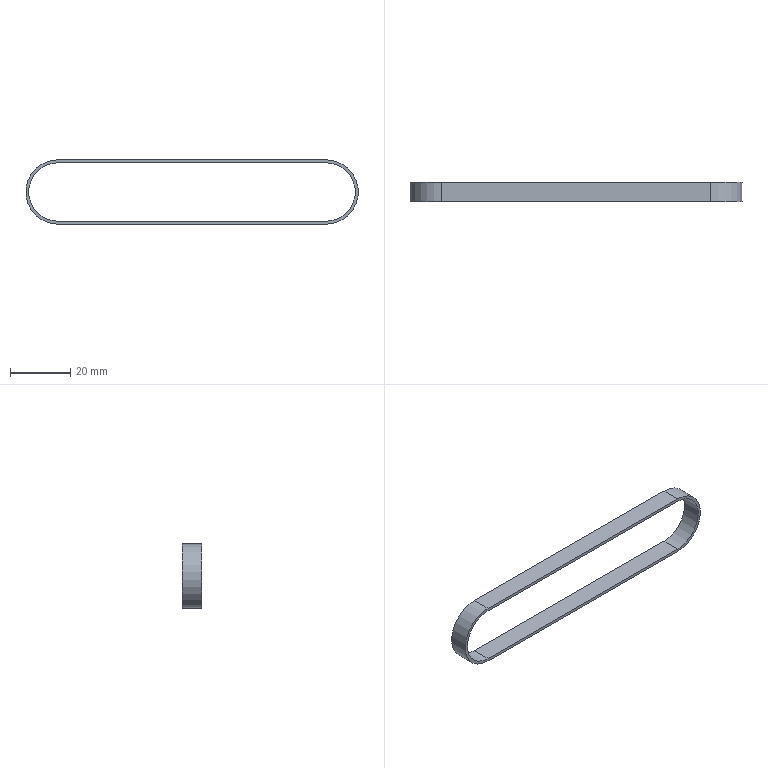Part | STEP file | MXL-025-118 | 1 solid | 10 faces | box 110.4 x 6.4 x 21.4 mm | volume 1549 mm3 | plane 6 | cylinder 4 | commonest cylinder face diameters 19.4 x2 21.4 x2
STEP:
#1=CARTESIAN_POINT('',(0.,0.,0.));
#2=DIRECTION('',(0.,0.,1.));
#3=DIRECTION('',(1.,0.,0.));
#4=AXIS2_PLACEMENT_3D('',#1,#2,#3);
#5=CARTESIAN_POINT('',(-42.816,6.4,-10.7));
#6=VERTEX_POINT('',#5);
#7=CARTESIAN_POINT('',(-42.816,6.4,10.7));
#8=VERTEX_POINT('',#7);
#9=CARTESIAN_POINT('',(-42.816,6.4,0.));
#10=DIRECTION('',(0.,1.,0.));
#11=DIRECTION('',(0.,0.,1.));
#12=AXIS2_PLACEMENT_3D('',#9,#10,#11);
#13=CIRCLE('',#12,10.7);
#14=CARTESIAN_POINT('',(-42.816,6.4,0.));
#15=DIRECTION('',(0.,1.,0.));
#16=DIRECTION('',(0.,0.,1.));
#17=AXIS2_PLACEMENT_3D('',#14,#15,#16);
#18=PLANE('',#17);
#19=CARTESIAN_POINT('',(0.,0.));
#20=DIRECTION('',(1.,0.));
#21=AXIS2_PLACEMENT_2D('',#19,#20);
#22=CIRCLE('',#21,10.7);
#23=(GEOMETRIC_REPRESENTATION_CONTEXT(2)PARAMETRIC_REPRESENTATION_CONTEXT()REPRESENTATION_CONTEXT('',''));
#24=DEFINITIONAL_REPRESENTATION('',(#22),#23);
#25=PCURVE('',#18,#24);
#26=CARTESIAN_POINT('',(-42.816,6.4,0.));
#27=DIRECTION('',(0.,-1.,0.));
#28=DIRECTION('',(0.,0.,-1.));
#29=AXIS2_PLACEMENT_3D('',#26,#27,#28);
#30=CYLINDRICAL_SURFACE('',#29,10.7);
#31=CARTESIAN_POINT('',(9.425,0.));
#32=DIRECTION('',(-1.,0.));
#33=VECTOR('',#32,1.);
#34=LINE('',#31,#33);
#35=(GEOMETRIC_REPRESENTATION_CONTEXT(2)PARAMETRIC_REPRESENTATION_CONTEXT()REPRESENTATION_CONTEXT('',''));
#36=DEFINITIONAL_REPRESENTATION('',(#34),#35);
#37=PCURVE('',#30,#36);
#38=SURFACE_CURVE('',#13,(#25,#37),.PCURVE_S1.);
#39=EDGE_CURVE('',#6,#8,#38,.T.);
#40=ORIENTED_EDGE('',*,*,#39,.T.);
#41=CARTESIAN_POINT('',(46.184,6.4,10.7));
#42=VERTEX_POINT('',#41);
#43=CARTESIAN_POINT('',(-42.816,6.4,10.7));
#44=DIRECTION('',(1.,0.,0.));
#45=VECTOR('',#44,1.);
#46=LINE('',#43,#45);
#47=CARTESIAN_POINT('',(10.7,0.));
#48=DIRECTION('',(0.,1.));
#49=VECTOR('',#48,1.);
#50=LINE('',#47,#49);
#51=(GEOMETRIC_REPRESENTATION_CONTEXT(2)PARAMETRIC_REPRESENTATION_CONTEXT()REPRESENTATION_CONTEXT('',''));
#52=DEFINITIONAL_REPRESENTATION('',(#50),#51);
#53=PCURVE('',#18,#52);
#54=CARTESIAN_POINT('',(-42.816,6.4,10.7));
#55=DIRECTION('',(0.,0.,-1.));
#56=DIRECTION('',(-1.,0.,0.));
#57=AXIS2_PLACEMENT_3D('',#54,#55,#56);
#58=PLANE('',#57);
#59=CARTESIAN_POINT('',(0.,0.));
#60=DIRECTION('',(-1.,0.));
#61=VECTOR('',#60,1.);
#62=LINE('',#59,#61);
#63=(GEOMETRIC_REPRESENTATION_CONTEXT(2)PARAMETRIC_REPRESENTATION_CONTEXT()REPRESENTATION_CONTEXT('',''));
#64=DEFINITIONAL_REPRESENTATION('',(#62),#63);
#65=PCURVE('',#58,#64);
#66=SURFACE_CURVE('',#46,(#53,#65),.PCURVE_S1.);
#67=EDGE_CURVE('',#8,#42,#66,.T.);
#68=ORIENTED_EDGE('',*,*,#67,.T.);
#69=CARTESIAN_POINT('',(46.184,6.4,-10.7));
#70=VERTEX_POINT('',#69);
#71=CARTESIAN_POINT('',(46.184,6.4,0.));
#72=DIRECTION('',(0.,1.,0.));
#73=DIRECTION('',(0.,0.,1.));
#74=AXIS2_PLACEMENT_3D('',#71,#72,#73);
#75=CIRCLE('',#74,10.7);
#76=CARTESIAN_POINT('',(0.,89.));
#77=DIRECTION('',(1.,0.));
#78=AXIS2_PLACEMENT_2D('',#76,#77);
#79=CIRCLE('',#78,10.7);
#80=(GEOMETRIC_REPRESENTATION_CONTEXT(2)PARAMETRIC_REPRESENTATION_CONTEXT()REPRESENTATION_CONTEXT('',''));
#81=DEFINITIONAL_REPRESENTATION('',(#79),#80);
#82=PCURVE('',#18,#81);
#83=CARTESIAN_POINT('',(46.184,6.4,0.));
#84=DIRECTION('',(0.,-1.,0.));
#85=DIRECTION('',(0.,0.,-1.));
#86=AXIS2_PLACEMENT_3D('',#83,#84,#85);
#87=CYLINDRICAL_SURFACE('',#86,10.7);
#88=CARTESIAN_POINT('',(3.142,0.));
#89=DIRECTION('',(-1.,0.));
#90=VECTOR('',#89,1.);
#91=LINE('',#88,#90);
#92=(GEOMETRIC_REPRESENTATION_CONTEXT(2)PARAMETRIC_REPRESENTATION_CONTEXT()REPRESENTATION_CONTEXT('',''));
#93=DEFINITIONAL_REPRESENTATION('',(#91),#92);
#94=PCURVE('',#87,#93);
#95=SURFACE_CURVE('',#75,(#82,#94),.PCURVE_S1.);
#96=EDGE_CURVE('',#42,#70,#95,.T.);
#97=ORIENTED_EDGE('',*,*,#96,.T.);
#98=CARTESIAN_POINT('',(-42.816,6.4,-10.7));
#99=DIRECTION('',(-1.,0.,0.));
#100=VECTOR('',#99,1.);
#101=LINE('',#98,#100);
#102=CARTESIAN_POINT('',(-10.7,0.));
#103=DIRECTION('',(0.,-1.));
#104=VECTOR('',#103,1.);
#105=LINE('',#102,#104);
#106=(GEOMETRIC_REPRESENTATION_CONTEXT(2)PARAMETRIC_REPRESENTATION_CONTEXT()REPRESENTATION_CONTEXT('',''));
#107=DEFINITIONAL_REPRESENTATION('',(#105),#106);
#108=PCURVE('',#18,#107);
#109=CARTESIAN_POINT('',(-42.816,6.4,-10.7));
#110=DIRECTION('',(0.,0.,1.));
#111=DIRECTION('',(1.,0.,0.));
#112=AXIS2_PLACEMENT_3D('',#109,#110,#111);
#113=PLANE('',#112);
#114=CARTESIAN_POINT('',(0.,0.));
#115=DIRECTION('',(-1.,0.));
#116=VECTOR('',#115,1.);
#117=LINE('',#114,#116);
#118=(GEOMETRIC_REPRESENTATION_CONTEXT(2)PARAMETRIC_REPRESENTATION_CONTEXT()REPRESENTATION_CONTEXT('',''));
#119=DEFINITIONAL_REPRESENTATION('',(#117),#118);
#120=PCURVE('',#113,#119);
#121=SURFACE_CURVE('',#101,(#108,#120),.PCURVE_S1.);
#122=EDGE_CURVE('',#70,#6,#121,.T.);
#123=ORIENTED_EDGE('',*,*,#122,.T.);
#124=EDGE_LOOP('',(#40,#68,#97,#123));
#125=FACE_BOUND('',#124,.T.);
#126=CARTESIAN_POINT('',(-42.816,6.4,9.7));
#127=VERTEX_POINT('',#126);
#128=CARTESIAN_POINT('',(46.184,6.4,9.7));
#129=VERTEX_POINT('',#128);
#130=CARTESIAN_POINT('',(-42.816,6.4,9.7));
#131=DIRECTION('',(1.,0.,0.));
#132=VECTOR('',#131,1.);
#133=LINE('',#130,#132);
#134=CARTESIAN_POINT('',(9.7,0.));
#135=DIRECTION('',(0.,1.));
#136=VECTOR('',#135,1.);
#137=LINE('',#134,#136);
#138=(GEOMETRIC_REPRESENTATION_CONTEXT(2)PARAMETRIC_REPRESENTATION_CONTEXT()REPRESENTATION_CONTEXT('',''));
#139=DEFINITIONAL_REPRESENTATION('',(#137),#138);
#140=PCURVE('',#18,#139);
#141=CARTESIAN_POINT('',(-42.816,6.4,9.7));
#142=DIRECTION('',(0.,0.,-1.));
#143=DIRECTION('',(-1.,0.,0.));
#144=AXIS2_PLACEMENT_3D('',#141,#142,#143);
#145=PLANE('',#144);
#146=CARTESIAN_POINT('',(0.,0.));
#147=DIRECTION('',(-1.,0.));
#148=VECTOR('',#147,1.);
#149=LINE('',#146,#148);
#150=(GEOMETRIC_REPRESENTATION_CONTEXT(2)PARAMETRIC_REPRESENTATION_CONTEXT()REPRESENTATION_CONTEXT('',''));
#151=DEFINITIONAL_REPRESENTATION('',(#149),#150);
#152=PCURVE('',#145,#151);
#153=SURFACE_CURVE('',#133,(#140,#152),.PCURVE_S1.);
#154=EDGE_CURVE('',#127,#129,#153,.T.);
#155=ORIENTED_EDGE('',*,*,#154,.F.);
#156=CARTESIAN_POINT('',(-42.816,6.4,-9.7));
#157=VERTEX_POINT('',#156);
#158=CARTESIAN_POINT('',(-42.816,6.4,0.));
#159=DIRECTION('',(0.,1.,0.));
#160=DIRECTION('',(0.,0.,1.));
#161=AXIS2_PLACEMENT_3D('',#158,#159,#160);
#162=CIRCLE('',#161,9.7);
#163=CARTESIAN_POINT('',(0.,0.));
#164=DIRECTION('',(1.,0.));
#165=AXIS2_PLACEMENT_2D('',#163,#164);
#166=CIRCLE('',#165,9.7);
#167=(GEOMETRIC_REPRESENTATION_CONTEXT(2)PARAMETRIC_REPRESENTATION_CONTEXT()REPRESENTATION_CONTEXT('',''));
#168=DEFINITIONAL_REPRESENTATION('',(#166),#167);
#169=PCURVE('',#18,#168);
#170=CARTESIAN_POINT('',(-42.816,6.4,0.));
#171=DIRECTION('',(0.,-1.,0.));
#172=DIRECTION('',(0.,0.,-1.));
#173=AXIS2_PLACEMENT_3D('',#170,#171,#172);
#174=CYLINDRICAL_SURFACE('',#173,9.7);
#175=CARTESIAN_POINT('',(9.425,0.));
#176=DIRECTION('',(-1.,0.));
#177=VECTOR('',#176,1.);
#178=LINE('',#175,#177);
#179=(GEOMETRIC_REPRESENTATION_CONTEXT(2)PARAMETRIC_REPRESENTATION_CONTEXT()REPRESENTATION_CONTEXT('',''));
#180=DEFINITIONAL_REPRESENTATION('',(#178),#179);
#181=PCURVE('',#174,#180);
#182=SURFACE_CURVE('',#162,(#169,#181),.PCURVE_S1.);
#183=EDGE_CURVE('',#157,#127,#182,.T.);
#184=ORIENTED_EDGE('',*,*,#183,.F.);
#185=CARTESIAN_POINT('',(46.184,6.4,-9.7));
#186=VERTEX_POINT('',#185);
#187=CARTESIAN_POINT('',(-42.816,6.4,-9.7));
#188=DIRECTION('',(-1.,0.,0.));
#189=VECTOR('',#188,1.);
#190=LINE('',#187,#189);
#191=CARTESIAN_POINT('',(-9.7,0.));
#192=DIRECTION('',(0.,-1.));
#193=VECTOR('',#192,1.);
#194=LINE('',#191,#193);
#195=(GEOMETRIC_REPRESENTATION_CONTEXT(2)PARAMETRIC_REPRESENTATION_CONTEXT()REPRESENTATION_CONTEXT('',''));
#196=DEFINITIONAL_REPRESENTATION('',(#194),#195);
#197=PCURVE('',#18,#196);
#198=CARTESIAN_POINT('',(-42.816,6.4,-9.7));
#199=DIRECTION('',(0.,0.,1.));
#200=DIRECTION('',(1.,0.,0.));
#201=AXIS2_PLACEMENT_3D('',#198,#199,#200);
#202=PLANE('',#201);
#203=CARTESIAN_POINT('',(0.,0.));
#204=DIRECTION('',(-1.,0.));
#205=VECTOR('',#204,1.);
#206=LINE('',#203,#205);
#207=(GEOMETRIC_REPRESENTATION_CONTEXT(2)PARAMETRIC_REPRESENTATION_CONTEXT()REPRESENTATION_CONTEXT('',''));
#208=DEFINITIONAL_REPRESENTATION('',(#206),#207);
#209=PCURVE('',#202,#208);
#210=SURFACE_CURVE('',#190,(#197,#209),.PCURVE_S1.);
#211=EDGE_CURVE('',#186,#157,#210,.T.);
#212=ORIENTED_EDGE('',*,*,#211,.F.);
#213=CARTESIAN_POINT('',(46.184,6.4,0.));
#214=DIRECTION('',(0.,1.,0.));
#215=DIRECTION('',(0.,0.,1.));
#216=AXIS2_PLACEMENT_3D('',#213,#214,#215);
#217=CIRCLE('',#216,9.7);
#218=CARTESIAN_POINT('',(0.,89.));
#219=DIRECTION('',(1.,0.));
#220=AXIS2_PLACEMENT_2D('',#218,#219);
#221=CIRCLE('',#220,9.7);
#222=(GEOMETRIC_REPRESENTATION_CONTEXT(2)PARAMETRIC_REPRESENTATION_CONTEXT()REPRESENTATION_CONTEXT('',''));
#223=DEFINITIONAL_REPRESENTATION('',(#221),#222);
#224=PCURVE('',#18,#223);
#225=CARTESIAN_POINT('',(46.184,6.4,0.));
#226=DIRECTION('',(0.,-1.,0.));
#227=DIRECTION('',(0.,0.,-1.));
#228=AXIS2_PLACEMENT_3D('',#225,#226,#227);
#229=CYLINDRICAL_SURFACE('',#228,9.7);
#230=CARTESIAN_POINT('',(3.142,0.));
#231=DIRECTION('',(-1.,0.));
#232=VECTOR('',#231,1.);
#233=LINE('',#230,#232);
#234=(GEOMETRIC_REPRESENTATION_CONTEXT(2)PARAMETRIC_REPRESENTATION_CONTEXT()REPRESENTATION_CONTEXT('',''));
#235=DEFINITIONAL_REPRESENTATION('',(#233),#234);
#236=PCURVE('',#229,#235);
#237=SURFACE_CURVE('',#217,(#224,#236),.PCURVE_S1.);
#238=EDGE_CURVE('',#129,#186,#237,.T.);
#239=ORIENTED_EDGE('',*,*,#238,.F.);
#240=EDGE_LOOP('',(#155,#184,#212,#239));
#241=FACE_BOUND('',#240,.T.);
#242=ADVANCED_FACE('',(#125,#241),#18,.T.);
#243=CARTESIAN_POINT('',(-42.816,0.,-10.7));
#244=VERTEX_POINT('',#243);
#245=CARTESIAN_POINT('',(-42.816,0.,10.7));
#246=VERTEX_POINT('',#245);
#247=CARTESIAN_POINT('',(-42.816,0.,0.));
#248=DIRECTION('',(0.,1.,0.));
#249=DIRECTION('',(0.,0.,1.));
#250=AXIS2_PLACEMENT_3D('',#247,#248,#249);
#251=CIRCLE('',#250,10.7);
#252=CARTESIAN_POINT('',(-42.816,0.,0.));
#253=DIRECTION('',(0.,1.,0.));
#254=DIRECTION('',(0.,0.,1.));
#255=AXIS2_PLACEMENT_3D('',#252,#253,#254);
#256=PLANE('',#255);
#257=CARTESIAN_POINT('',(0.,0.));
#258=DIRECTION('',(1.,0.));
#259=AXIS2_PLACEMENT_2D('',#257,#258);
#260=CIRCLE('',#259,10.7);
#261=(GEOMETRIC_REPRESENTATION_CONTEXT(2)PARAMETRIC_REPRESENTATION_CONTEXT()REPRESENTATION_CONTEXT('',''));
#262=DEFINITIONAL_REPRESENTATION('',(#260),#261);
#263=PCURVE('',#256,#262);
#264=CARTESIAN_POINT('',(9.425,6.4));
#265=DIRECTION('',(-1.,0.));
#266=VECTOR('',#265,1.);
#267=LINE('',#264,#266);
#268=(GEOMETRIC_REPRESENTATION_CONTEXT(2)PARAMETRIC_REPRESENTATION_CONTEXT()REPRESENTATION_CONTEXT('',''));
#269=DEFINITIONAL_REPRESENTATION('',(#267),#268);
#270=PCURVE('',#30,#269);
#271=SURFACE_CURVE('',#251,(#263,#270),.PCURVE_S1.);
#272=EDGE_CURVE('',#244,#246,#271,.T.);
#273=ORIENTED_EDGE('',*,*,#272,.F.);
#274=CARTESIAN_POINT('',(46.184,0.,-10.7));
#275=VERTEX_POINT('',#274);
#276=CARTESIAN_POINT('',(-42.816,0.,-10.7));
#277=DIRECTION('',(-1.,0.,0.));
#278=VECTOR('',#277,1.);
#279=LINE('',#276,#278);
#280=CARTESIAN_POINT('',(-10.7,0.));
#281=DIRECTION('',(0.,-1.));
#282=VECTOR('',#281,1.);
#283=LINE('',#280,#282);
#284=(GEOMETRIC_REPRESENTATION_CONTEXT(2)PARAMETRIC_REPRESENTATION_CONTEXT()REPRESENTATION_CONTEXT('',''));
#285=DEFINITIONAL_REPRESENTATION('',(#283),#284);
#286=PCURVE('',#256,#285);
#287=CARTESIAN_POINT('',(0.,-6.4));
#288=DIRECTION('',(-1.,0.));
#289=VECTOR('',#288,1.);
#290=LINE('',#287,#289);
#291=(GEOMETRIC_REPRESENTATION_CONTEXT(2)PARAMETRIC_REPRESENTATION_CONTEXT()REPRESENTATION_CONTEXT('',''));
#292=DEFINITIONAL_REPRESENTATION('',(#290),#291);
#293=PCURVE('',#113,#292);
#294=SURFACE_CURVE('',#279,(#286,#293),.PCURVE_S1.);
#295=EDGE_CURVE('',#275,#244,#294,.T.);
#296=ORIENTED_EDGE('',*,*,#295,.F.);
#297=CARTESIAN_POINT('',(46.184,0.,10.7));
#298=VERTEX_POINT('',#297);
#299=CARTESIAN_POINT('',(46.184,0.,0.));
#300=DIRECTION('',(0.,1.,0.));
#301=DIRECTION('',(0.,0.,1.));
#302=AXIS2_PLACEMENT_3D('',#299,#300,#301);
#303=CIRCLE('',#302,10.7);
#304=CARTESIAN_POINT('',(0.,89.));
#305=DIRECTION('',(1.,0.));
#306=AXIS2_PLACEMENT_2D('',#304,#305);
#307=CIRCLE('',#306,10.7);
#308=(GEOMETRIC_REPRESENTATION_CONTEXT(2)PARAMETRIC_REPRESENTATION_CONTEXT()REPRESENTATION_CONTEXT('',''));
#309=DEFINITIONAL_REPRESENTATION('',(#307),#308);
#310=PCURVE('',#256,#309);
#311=CARTESIAN_POINT('',(3.142,6.4));
#312=DIRECTION('',(-1.,0.));
#313=VECTOR('',#312,1.);
#314=LINE('',#311,#313);
#315=(GEOMETRIC_REPRESENTATION_CONTEXT(2)PARAMETRIC_REPRESENTATION_CONTEXT()REPRESENTATION_CONTEXT('',''));
#316=DEFINITIONAL_REPRESENTATION('',(#314),#315);
#317=PCURVE('',#87,#316);
#318=SURFACE_CURVE('',#303,(#310,#317),.PCURVE_S1.);
#319=EDGE_CURVE('',#298,#275,#318,.T.);
#320=ORIENTED_EDGE('',*,*,#319,.F.);
#321=CARTESIAN_POINT('',(-42.816,0.,10.7));
#322=DIRECTION('',(1.,0.,0.));
#323=VECTOR('',#322,1.);
#324=LINE('',#321,#323);
#325=CARTESIAN_POINT('',(10.7,0.));
#326=DIRECTION('',(0.,1.));
#327=VECTOR('',#326,1.);
#328=LINE('',#325,#327);
#329=(GEOMETRIC_REPRESENTATION_CONTEXT(2)PARAMETRIC_REPRESENTATION_CONTEXT()REPRESENTATION_CONTEXT('',''));
#330=DEFINITIONAL_REPRESENTATION('',(#328),#329);
#331=PCURVE('',#256,#330);
#332=CARTESIAN_POINT('',(0.,-6.4));
#333=DIRECTION('',(-1.,0.));
#334=VECTOR('',#333,1.);
#335=LINE('',#332,#334);
#336=(GEOMETRIC_REPRESENTATION_CONTEXT(2)PARAMETRIC_REPRESENTATION_CONTEXT()REPRESENTATION_CONTEXT('',''));
#337=DEFINITIONAL_REPRESENTATION('',(#335),#336);
#338=PCURVE('',#58,#337);
#339=SURFACE_CURVE('',#324,(#331,#338),.PCURVE_S1.);
#340=EDGE_CURVE('',#246,#298,#339,.T.);
#341=ORIENTED_EDGE('',*,*,#340,.F.);
#342=EDGE_LOOP('',(#273,#296,#320,#341));
#343=FACE_BOUND('',#342,.T.);
#344=CARTESIAN_POINT('',(-42.816,0.,-9.7));
#345=VERTEX_POINT('',#344);
#346=CARTESIAN_POINT('',(-42.816,0.,9.7));
#347=VERTEX_POINT('',#346);
#348=CARTESIAN_POINT('',(-42.816,0.,0.));
#349=DIRECTION('',(0.,1.,0.));
#350=DIRECTION('',(0.,0.,1.));
#351=AXIS2_PLACEMENT_3D('',#348,#349,#350);
#352=CIRCLE('',#351,9.7);
#353=CARTESIAN_POINT('',(0.,0.));
#354=DIRECTION('',(1.,0.));
#355=AXIS2_PLACEMENT_2D('',#353,#354);
#356=CIRCLE('',#355,9.7);
#357=(GEOMETRIC_REPRESENTATION_CONTEXT(2)PARAMETRIC_REPRESENTATION_CONTEXT()REPRESENTATION_CONTEXT('',''));
#358=DEFINITIONAL_REPRESENTATION('',(#356),#357);
#359=PCURVE('',#256,#358);
#360=CARTESIAN_POINT('',(9.425,6.4));
#361=DIRECTION('',(-1.,0.));
#362=VECTOR('',#361,1.);
#363=LINE('',#360,#362);
#364=(GEOMETRIC_REPRESENTATION_CONTEXT(2)PARAMETRIC_REPRESENTATION_CONTEXT()REPRESENTATION_CONTEXT('',''));
#365=DEFINITIONAL_REPRESENTATION('',(#363),#364);
#366=PCURVE('',#174,#365);
#367=SURFACE_CURVE('',#352,(#359,#366),.PCURVE_S1.);
#368=EDGE_CURVE('',#345,#347,#367,.T.);
#369=ORIENTED_EDGE('',*,*,#368,.T.);
#370=CARTESIAN_POINT('',(46.184,0.,9.7));
#371=VERTEX_POINT('',#370);
#372=CARTESIAN_POINT('',(-42.816,0.,9.7));
#373=DIRECTION('',(1.,0.,0.));
#374=VECTOR('',#373,1.);
#375=LINE('',#372,#374);
#376=CARTESIAN_POINT('',(9.7,0.));
#377=DIRECTION('',(0.,1.));
#378=VECTOR('',#377,1.);
#379=LINE('',#376,#378);
#380=(GEOMETRIC_REPRESENTATION_CONTEXT(2)PARAMETRIC_REPRESENTATION_CONTEXT()REPRESENTATION_CONTEXT('',''));
#381=DEFINITIONAL_REPRESENTATION('',(#379),#380);
#382=PCURVE('',#256,#381);
#383=CARTESIAN_POINT('',(0.,-6.4));
#384=DIRECTION('',(-1.,0.));
#385=VECTOR('',#384,1.);
#386=LINE('',#383,#385);
#387=(GEOMETRIC_REPRESENTATION_CONTEXT(2)PARAMETRIC_REPRESENTATION_CONTEXT()REPRESENTATION_CONTEXT('',''));
#388=DEFINITIONAL_REPRESENTATION('',(#386),#387);
#389=PCURVE('',#145,#388);
#390=SURFACE_CURVE('',#375,(#382,#389),.PCURVE_S1.);
#391=EDGE_CURVE('',#347,#371,#390,.T.);
#392=ORIENTED_EDGE('',*,*,#391,.T.);
#393=CARTESIAN_POINT('',(46.184,0.,-9.7));
#394=VERTEX_POINT('',#393);
#395=CARTESIAN_POINT('',(46.184,0.,0.));
#396=DIRECTION('',(0.,1.,0.));
#397=DIRECTION('',(0.,0.,1.));
#398=AXIS2_PLACEMENT_3D('',#395,#396,#397);
#399=CIRCLE('',#398,9.7);
#400=CARTESIAN_POINT('',(0.,89.));
#401=DIRECTION('',(1.,0.));
#402=AXIS2_PLACEMENT_2D('',#400,#401);
#403=CIRCLE('',#402,9.7);
#404=(GEOMETRIC_REPRESENTATION_CONTEXT(2)PARAMETRIC_REPRESENTATION_CONTEXT()REPRESENTATION_CONTEXT('',''));
#405=DEFINITIONAL_REPRESENTATION('',(#403),#404);
#406=PCURVE('',#256,#405);
#407=CARTESIAN_POINT('',(3.142,6.4));
#408=DIRECTION('',(-1.,0.));
#409=VECTOR('',#408,1.);
#410=LINE('',#407,#409);
#411=(GEOMETRIC_REPRESENTATION_CONTEXT(2)PARAMETRIC_REPRESENTATION_CONTEXT()REPRESENTATION_CONTEXT('',''));
#412=DEFINITIONAL_REPRESENTATION('',(#410),#411);
#413=PCURVE('',#229,#412);
#414=SURFACE_CURVE('',#399,(#406,#413),.PCURVE_S1.);
#415=EDGE_CURVE('',#371,#394,#414,.T.);
#416=ORIENTED_EDGE('',*,*,#415,.T.);
#417=CARTESIAN_POINT('',(-42.816,0.,-9.7));
#418=DIRECTION('',(-1.,0.,0.));
#419=VECTOR('',#418,1.);
#420=LINE('',#417,#419);
#421=CARTESIAN_POINT('',(-9.7,0.));
#422=DIRECTION('',(0.,-1.));
#423=VECTOR('',#422,1.);
#424=LINE('',#421,#423);
#425=(GEOMETRIC_REPRESENTATION_CONTEXT(2)PARAMETRIC_REPRESENTATION_CONTEXT()REPRESENTATION_CONTEXT('',''));
#426=DEFINITIONAL_REPRESENTATION('',(#424),#425);
#427=PCURVE('',#256,#426);
#428=CARTESIAN_POINT('',(0.,-6.4));
#429=DIRECTION('',(-1.,0.));
#430=VECTOR('',#429,1.);
#431=LINE('',#428,#430);
#432=(GEOMETRIC_REPRESENTATION_CONTEXT(2)PARAMETRIC_REPRESENTATION_CONTEXT()REPRESENTATION_CONTEXT('',''));
#433=DEFINITIONAL_REPRESENTATION('',(#431),#432);
#434=PCURVE('',#202,#433);
#435=SURFACE_CURVE('',#420,(#427,#434),.PCURVE_S1.);
#436=EDGE_CURVE('',#394,#345,#435,.T.);
#437=ORIENTED_EDGE('',*,*,#436,.T.);
#438=EDGE_LOOP('',(#369,#392,#416,#437));
#439=FACE_BOUND('',#438,.T.);
#440=ADVANCED_FACE('',(#343,#439),#256,.F.);
#441=ORIENTED_EDGE('',*,*,#272,.T.);
#442=CARTESIAN_POINT('',(-42.816,6.4,10.7));
#443=DIRECTION('',(0.,-1.,0.));
#444=VECTOR('',#443,1.);
#445=LINE('',#442,#444);
#446=CARTESIAN_POINT('',(3.142,0.));
#447=DIRECTION('',(0.,1.));
#448=VECTOR('',#447,1.);
#449=LINE('',#446,#448);
#450=(GEOMETRIC_REPRESENTATION_CONTEXT(2)PARAMETRIC_REPRESENTATION_CONTEXT()REPRESENTATION_CONTEXT('',''));
#451=DEFINITIONAL_REPRESENTATION('',(#449),#450);
#452=PCURVE('',#30,#451);
#453=CARTESIAN_POINT('',(0.,0.));
#454=DIRECTION('',(0.,-1.));
#455=VECTOR('',#454,1.);
#456=LINE('',#453,#455);
#457=(GEOMETRIC_REPRESENTATION_CONTEXT(2)PARAMETRIC_REPRESENTATION_CONTEXT()REPRESENTATION_CONTEXT('',''));
#458=DEFINITIONAL_REPRESENTATION('',(#456),#457);
#459=PCURVE('',#58,#458);
#460=SURFACE_CURVE('',#445,(#452,#459),.PCURVE_S1.);
#461=EDGE_CURVE('',#8,#246,#460,.T.);
#462=ORIENTED_EDGE('',*,*,#461,.F.);
#463=ORIENTED_EDGE('',*,*,#39,.F.);
#464=CARTESIAN_POINT('',(-42.816,6.4,-10.7));
#465=DIRECTION('',(0.,-1.,0.));
#466=VECTOR('',#465,1.);
#467=LINE('',#464,#466);
#468=CARTESIAN_POINT('',(6.283,0.));
#469=DIRECTION('',(0.,1.));
#470=VECTOR('',#469,1.);
#471=LINE('',#468,#470);
#472=(GEOMETRIC_REPRESENTATION_CONTEXT(2)PARAMETRIC_REPRESENTATION_CONTEXT()REPRESENTATION_CONTEXT('',''));
#473=DEFINITIONAL_REPRESENTATION('',(#471),#472);
#474=PCURVE('',#30,#473);
#475=CARTESIAN_POINT('',(0.,0.));
#476=DIRECTION('',(0.,-1.));
#477=VECTOR('',#476,1.);
#478=LINE('',#475,#477);
#479=(GEOMETRIC_REPRESENTATION_CONTEXT(2)PARAMETRIC_REPRESENTATION_CONTEXT()REPRESENTATION_CONTEXT('',''));
#480=DEFINITIONAL_REPRESENTATION('',(#478),#479);
#481=PCURVE('',#113,#480);
#482=SURFACE_CURVE('',#467,(#474,#481),.PCURVE_S1.);
#483=EDGE_CURVE('',#6,#244,#482,.T.);
#484=ORIENTED_EDGE('',*,*,#483,.T.);
#485=EDGE_LOOP('',(#441,#462,#463,#484));
#486=FACE_BOUND('',#485,.T.);
#487=ADVANCED_FACE('',(#486),#30,.T.);
#488=ORIENTED_EDGE('',*,*,#340,.T.);
#489=CARTESIAN_POINT('',(46.184,6.4,10.7));
#490=DIRECTION('',(0.,-1.,0.));
#491=VECTOR('',#490,1.);
#492=LINE('',#489,#491);
#493=CARTESIAN_POINT('',(-89.,0.));
#494=DIRECTION('',(0.,-1.));
#495=VECTOR('',#494,1.);
#496=LINE('',#493,#495);
#497=(GEOMETRIC_REPRESENTATION_CONTEXT(2)PARAMETRIC_REPRESENTATION_CONTEXT()REPRESENTATION_CONTEXT('',''));
#498=DEFINITIONAL_REPRESENTATION('',(#496),#497);
#499=PCURVE('',#58,#498);
#500=CARTESIAN_POINT('',(3.142,0.));
#501=DIRECTION('',(0.,1.));
#502=VECTOR('',#501,1.);
#503=LINE('',#500,#502);
#504=(GEOMETRIC_REPRESENTATION_CONTEXT(2)PARAMETRIC_REPRESENTATION_CONTEXT()REPRESENTATION_CONTEXT('',''));
#505=DEFINITIONAL_REPRESENTATION('',(#503),#504);
#506=PCURVE('',#87,#505);
#507=SURFACE_CURVE('',#492,(#499,#506),.PCURVE_S1.);
#508=EDGE_CURVE('',#42,#298,#507,.T.);
#509=ORIENTED_EDGE('',*,*,#508,.F.);
#510=ORIENTED_EDGE('',*,*,#67,.F.);
#511=ORIENTED_EDGE('',*,*,#461,.T.);
#512=EDGE_LOOP('',(#488,#509,#510,#511));
#513=FACE_BOUND('',#512,.T.);
#514=ADVANCED_FACE('',(#513),#58,.F.);
#515=ORIENTED_EDGE('',*,*,#319,.T.);
#516=CARTESIAN_POINT('',(46.184,6.4,-10.7));
#517=DIRECTION('',(0.,-1.,0.));
#518=VECTOR('',#517,1.);
#519=LINE('',#516,#518);
#520=CARTESIAN_POINT('',(0.,0.));
#521=DIRECTION('',(0.,1.));
#522=VECTOR('',#521,1.);
#523=LINE('',#520,#522);
#524=(GEOMETRIC_REPRESENTATION_CONTEXT(2)PARAMETRIC_REPRESENTATION_CONTEXT()REPRESENTATION_CONTEXT('',''));
#525=DEFINITIONAL_REPRESENTATION('',(#523),#524);
#526=PCURVE('',#87,#525);
#527=CARTESIAN_POINT('',(89.,0.));
#528=DIRECTION('',(0.,-1.));
#529=VECTOR('',#528,1.);
#530=LINE('',#527,#529);
#531=(GEOMETRIC_REPRESENTATION_CONTEXT(2)PARAMETRIC_REPRESENTATION_CONTEXT()REPRESENTATION_CONTEXT('',''));
#532=DEFINITIONAL_REPRESENTATION('',(#530),#531);
#533=PCURVE('',#113,#532);
#534=SURFACE_CURVE('',#519,(#526,#533),.PCURVE_S1.);
#535=EDGE_CURVE('',#70,#275,#534,.T.);
#536=ORIENTED_EDGE('',*,*,#535,.F.);
#537=ORIENTED_EDGE('',*,*,#96,.F.);
#538=ORIENTED_EDGE('',*,*,#508,.T.);
#539=EDGE_LOOP('',(#515,#536,#537,#538));
#540=FACE_BOUND('',#539,.T.);
#541=ADVANCED_FACE('',(#540),#87,.T.);
#542=ORIENTED_EDGE('',*,*,#295,.T.);
#543=ORIENTED_EDGE('',*,*,#483,.F.);
#544=ORIENTED_EDGE('',*,*,#122,.F.);
#545=ORIENTED_EDGE('',*,*,#535,.T.);
#546=EDGE_LOOP('',(#542,#543,#544,#545));
#547=FACE_BOUND('',#546,.T.);
#548=ADVANCED_FACE('',(#547),#113,.F.);
#549=CARTESIAN_POINT('',(-42.816,6.4,9.7));
#550=DIRECTION('',(0.,-1.,0.));
#551=VECTOR('',#550,1.);
#552=LINE('',#549,#551);
#553=CARTESIAN_POINT('',(3.142,0.));
#554=DIRECTION('',(0.,1.));
#555=VECTOR('',#554,1.);
#556=LINE('',#553,#555);
#557=(GEOMETRIC_REPRESENTATION_CONTEXT(2)PARAMETRIC_REPRESENTATION_CONTEXT()REPRESENTATION_CONTEXT('',''));
#558=DEFINITIONAL_REPRESENTATION('',(#556),#557);
#559=PCURVE('',#174,#558);
#560=CARTESIAN_POINT('',(0.,0.));
#561=DIRECTION('',(0.,-1.));
#562=VECTOR('',#561,1.);
#563=LINE('',#560,#562);
#564=(GEOMETRIC_REPRESENTATION_CONTEXT(2)PARAMETRIC_REPRESENTATION_CONTEXT()REPRESENTATION_CONTEXT('',''));
#565=DEFINITIONAL_REPRESENTATION('',(#563),#564);
#566=PCURVE('',#145,#565);
#567=SURFACE_CURVE('',#552,(#559,#566),.PCURVE_S1.);
#568=EDGE_CURVE('',#127,#347,#567,.T.);
#569=ORIENTED_EDGE('',*,*,#568,.F.);
#570=ORIENTED_EDGE('',*,*,#183,.F.);
#571=CARTESIAN_POINT('',(-42.816,6.4,-9.7));
#572=DIRECTION('',(0.,-1.,0.));
#573=VECTOR('',#572,1.);
#574=LINE('',#571,#573);
#575=CARTESIAN_POINT('',(6.283,0.));
#576=DIRECTION('',(0.,1.));
#577=VECTOR('',#576,1.);
#578=LINE('',#575,#577);
#579=(GEOMETRIC_REPRESENTATION_CONTEXT(2)PARAMETRIC_REPRESENTATION_CONTEXT()REPRESENTATION_CONTEXT('',''));
#580=DEFINITIONAL_REPRESENTATION('',(#578),#579);
#581=PCURVE('',#174,#580);
#582=CARTESIAN_POINT('',(0.,0.));
#583=DIRECTION('',(0.,-1.));
#584=VECTOR('',#583,1.);
#585=LINE('',#582,#584);
#586=(GEOMETRIC_REPRESENTATION_CONTEXT(2)PARAMETRIC_REPRESENTATION_CONTEXT()REPRESENTATION_CONTEXT('',''));
#587=DEFINITIONAL_REPRESENTATION('',(#585),#586);
#588=PCURVE('',#202,#587);
#589=SURFACE_CURVE('',#574,(#581,#588),.PCURVE_S1.);
#590=EDGE_CURVE('',#157,#345,#589,.T.);
#591=ORIENTED_EDGE('',*,*,#590,.T.);
#592=ORIENTED_EDGE('',*,*,#368,.T.);
#593=EDGE_LOOP('',(#569,#570,#591,#592));
#594=FACE_BOUND('',#593,.F.);
#595=ADVANCED_FACE('',(#594),#174,.F.);
#596=ORIENTED_EDGE('',*,*,#391,.F.);
#597=ORIENTED_EDGE('',*,*,#568,.F.);
#598=ORIENTED_EDGE('',*,*,#154,.T.);
#599=CARTESIAN_POINT('',(46.184,6.4,9.7));
#600=DIRECTION('',(0.,-1.,0.));
#601=VECTOR('',#600,1.);
#602=LINE('',#599,#601);
#603=CARTESIAN_POINT('',(-89.,0.));
#604=DIRECTION('',(0.,-1.));
#605=VECTOR('',#604,1.);
#606=LINE('',#603,#605);
#607=(GEOMETRIC_REPRESENTATION_CONTEXT(2)PARAMETRIC_REPRESENTATION_CONTEXT()REPRESENTATION_CONTEXT('',''));
#608=DEFINITIONAL_REPRESENTATION('',(#606),#607);
#609=PCURVE('',#145,#608);
#610=CARTESIAN_POINT('',(3.142,0.));
#611=DIRECTION('',(0.,1.));
#612=VECTOR('',#611,1.);
#613=LINE('',#610,#612);
#614=(GEOMETRIC_REPRESENTATION_CONTEXT(2)PARAMETRIC_REPRESENTATION_CONTEXT()REPRESENTATION_CONTEXT('',''));
#615=DEFINITIONAL_REPRESENTATION('',(#613),#614);
#616=PCURVE('',#229,#615);
#617=SURFACE_CURVE('',#602,(#609,#616),.PCURVE_S1.);
#618=EDGE_CURVE('',#129,#371,#617,.T.);
#619=ORIENTED_EDGE('',*,*,#618,.T.);
#620=EDGE_LOOP('',(#596,#597,#598,#619));
#621=FACE_BOUND('',#620,.T.);
#622=ADVANCED_FACE('',(#621),#145,.T.);
#623=CARTESIAN_POINT('',(46.184,6.4,-9.7));
#624=DIRECTION('',(0.,-1.,0.));
#625=VECTOR('',#624,1.);
#626=LINE('',#623,#625);
#627=CARTESIAN_POINT('',(0.,0.));
#628=DIRECTION('',(0.,1.));
#629=VECTOR('',#628,1.);
#630=LINE('',#627,#629);
#631=(GEOMETRIC_REPRESENTATION_CONTEXT(2)PARAMETRIC_REPRESENTATION_CONTEXT()REPRESENTATION_CONTEXT('',''));
#632=DEFINITIONAL_REPRESENTATION('',(#630),#631);
#633=PCURVE('',#229,#632);
#634=CARTESIAN_POINT('',(89.,0.));
#635=DIRECTION('',(0.,-1.));
#636=VECTOR('',#635,1.);
#637=LINE('',#634,#636);
#638=(GEOMETRIC_REPRESENTATION_CONTEXT(2)PARAMETRIC_REPRESENTATION_CONTEXT()REPRESENTATION_CONTEXT('',''));
#639=DEFINITIONAL_REPRESENTATION('',(#637),#638);
#640=PCURVE('',#202,#639);
#641=SURFACE_CURVE('',#626,(#633,#640),.PCURVE_S1.);
#642=EDGE_CURVE('',#186,#394,#641,.T.);
#643=ORIENTED_EDGE('',*,*,#642,.F.);
#644=ORIENTED_EDGE('',*,*,#238,.F.);
#645=ORIENTED_EDGE('',*,*,#618,.T.);
#646=ORIENTED_EDGE('',*,*,#415,.T.);
#647=EDGE_LOOP('',(#643,#644,#645,#646));
#648=FACE_BOUND('',#647,.F.);
#649=ADVANCED_FACE('',(#648),#229,.F.);
#650=ORIENTED_EDGE('',*,*,#436,.F.);
#651=ORIENTED_EDGE('',*,*,#642,.F.);
#652=ORIENTED_EDGE('',*,*,#211,.T.);
#653=ORIENTED_EDGE('',*,*,#590,.T.);
#654=EDGE_LOOP('',(#650,#651,#652,#653));
#655=FACE_BOUND('',#654,.T.);
#656=ADVANCED_FACE('',(#655),#202,.T.);
#657=CLOSED_SHELL('',(#242,#440,#487,#514,#541,#548,#595,#622,#649,#656));
#658=MANIFOLD_SOLID_BREP('',#657);
#659=(LENGTH_UNIT()NAMED_UNIT(*)SI_UNIT(.MILLI.,.METRE.));
#660=UNCERTAINTY_MEASURE_WITH_UNIT(LENGTH_MEASURE(0.0000001),#659,'','');
#661=(NAMED_UNIT(*)PLANE_ANGLE_UNIT()SI_UNIT($,.RADIAN.));
#662=(NAMED_UNIT(*)SI_UNIT($,.STERADIAN.)SOLID_ANGLE_UNIT());
#663=(GEOMETRIC_REPRESENTATION_CONTEXT(3)GLOBAL_UNCERTAINTY_ASSIGNED_CONTEXT((#660))GLOBAL_UNIT_ASSIGNED_CONTEXT((#659,#661,#662))REPRESENTATION_CONTEXT('',''));
#664=ADVANCED_BREP_SHAPE_REPRESENTATION('',(#4,#658),#663);